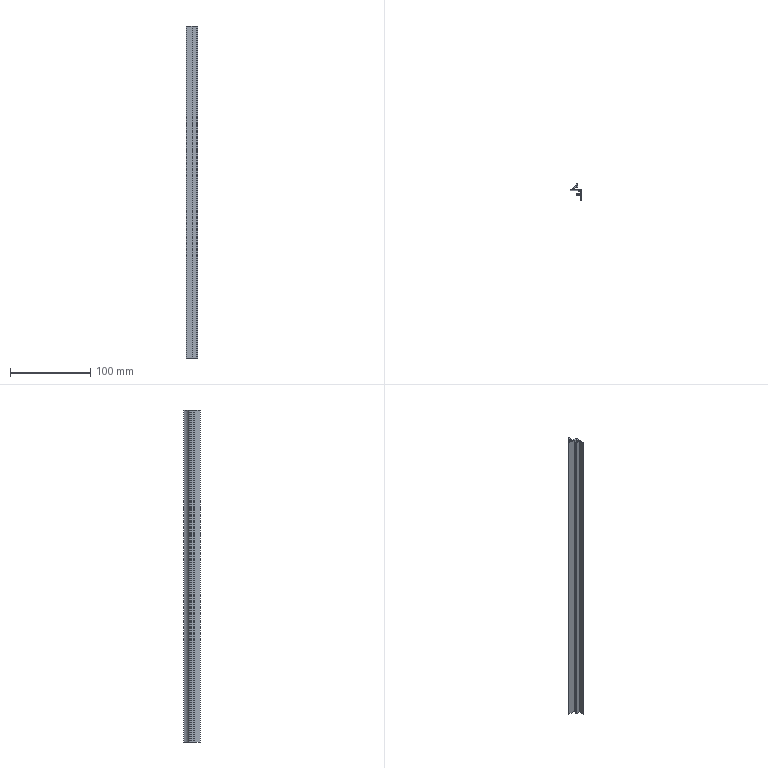Part | SolidWorks | features BaseBody 1, ICE 1, MoveFace 1 | 1 solid | 27 faces | box 14 x 20.3 x 413 mm | volume 21028 mm3 | plane 20 | cylinder 7 | commonest cylinder face diameters 0.387 x2 0.8 x2 0.4 x1 20 x1 22 x1
STEP:
#1=CARTESIAN_POINT('',(-5.304,-0.625,200.));
#2=VERTEX_POINT('',#1);
#3=CARTESIAN_POINT('',(-5.449,-0.8125,200.));
#4=VERTEX_POINT('',#3);
#5=CARTESIAN_POINT('',(-5.255,-0.8125,200.));
#6=DIRECTION('',(0.,0.,1.));
#7=DIRECTION('',(-1.,0.,0.));
#8=AXIS2_PLACEMENT_3D('',#5,#6,#7);
#9=CIRCLE('',#8,0.1937);
#10=EDGE_CURVE('',#2,#4,#9,.T.);
#11=ORIENTED_EDGE('',*,*,#10,.T.);
#12=CARTESIAN_POINT('',(-5.449,-0.8125,-213.));
#13=VERTEX_POINT('',#12);
#14=CARTESIAN_POINT('',(-5.449,-0.8125,230.));
#15=DIRECTION('',(0.,0.,-1.));
#16=VECTOR('',#15,1000.);
#17=LINE('',#14,#16);
#18=EDGE_CURVE('',#4,#13,#17,.T.);
#19=ORIENTED_EDGE('',*,*,#18,.T.);
#20=CARTESIAN_POINT('',(-5.304,-0.625,-213.));
#21=VERTEX_POINT('',#20);
#22=CARTESIAN_POINT('',(-5.255,-0.8125,-213.));
#23=DIRECTION('',(0.,0.,-1.));
#24=DIRECTION('',(1.,0.,0.));
#25=AXIS2_PLACEMENT_3D('',#22,#23,#24);
#26=CIRCLE('',#25,0.1937);
#27=EDGE_CURVE('',#13,#21,#26,.T.);
#28=ORIENTED_EDGE('',*,*,#27,.T.);
#29=CARTESIAN_POINT('',(-5.304,-0.625,230.));
#30=DIRECTION('',(0.,0.,-1.));
#31=VECTOR('',#30,1000.);
#32=LINE('',#29,#31);
#33=EDGE_CURVE('',#2,#21,#32,.T.);
#34=ORIENTED_EDGE('',*,*,#33,.F.);
#35=EDGE_LOOP('',(#11,#19,#28,#34));
#36=FACE_OUTER_BOUND('',#35,.T.);
#37=CARTESIAN_POINT('',(-5.255,-0.8125,230.));
#38=DIRECTION('',(0.,0.,-1.));
#39=DIRECTION('',(-1.,0.,0.));
#40=AXIS2_PLACEMENT_3D('',#37,#38,#39);
#41=CYLINDRICAL_SURFACE('',#40,0.1937);
#42=ADVANCED_FACE('',(#36),#41,.F.);
#43=CARTESIAN_POINT('',(5.,-1.,-213.));
#44=VERTEX_POINT('',#43);
#45=CARTESIAN_POINT('',(5.,-14.3,-213.));
#46=VERTEX_POINT('',#45);
#47=CARTESIAN_POINT('',(5.,29.623,-213.));
#48=DIRECTION('',(0.,-1.,0.));
#49=VECTOR('',#48,1000.);
#50=LINE('',#47,#49);
#51=EDGE_CURVE('',#44,#46,#50,.T.);
#52=ORIENTED_EDGE('',*,*,#51,.F.);
#53=CARTESIAN_POINT('',(5.,-1.,200.));
#54=VERTEX_POINT('',#53);
#55=CARTESIAN_POINT('',(5.,-1.,230.));
#56=DIRECTION('',(0.,0.,-1.));
#57=VECTOR('',#56,1000.);
#58=LINE('',#55,#57);
#59=EDGE_CURVE('',#54,#44,#58,.T.);
#60=ORIENTED_EDGE('',*,*,#59,.F.);
#61=CARTESIAN_POINT('',(5.,-14.3,200.));
#62=VERTEX_POINT('',#61);
#63=CARTESIAN_POINT('',(5.,-14.3,200.));
#64=DIRECTION('',(0.,1.,0.));
#65=VECTOR('',#64,1000.);
#66=LINE('',#63,#65);
#67=EDGE_CURVE('',#62,#54,#66,.T.);
#68=ORIENTED_EDGE('',*,*,#67,.F.);
#69=CARTESIAN_POINT('',(5.,-14.3,230.));
#70=DIRECTION('',(0.,0.,1.));
#71=VECTOR('',#70,1000.);
#72=LINE('',#69,#71);
#73=EDGE_CURVE('',#46,#62,#72,.T.);
#74=ORIENTED_EDGE('',*,*,#73,.F.);
#75=EDGE_LOOP('',(#52,#60,#68,#74));
#76=FACE_OUTER_BOUND('',#75,.T.);
#77=CARTESIAN_POINT('',(5.,-14.3,230.));
#78=DIRECTION('',(-1.,0.,0.));
#79=DIRECTION('',(0.,0.,1.));
#80=AXIS2_PLACEMENT_3D('',#77,#78,#79);
#81=PLANE('',#80);
#82=ADVANCED_FACE('',(#76),#81,.F.);
#83=CARTESIAN_POINT('',(-9.,-2.,-213.));
#84=VERTEX_POINT('',#83);
#85=CARTESIAN_POINT('',(-9.,-2.,200.));
#86=VERTEX_POINT('',#85);
#87=CARTESIAN_POINT('',(-9.,-2.,230.));
#88=DIRECTION('',(0.,0.,1.));
#89=VECTOR('',#88,1000.);
#90=LINE('',#87,#89);
#91=EDGE_CURVE('',#84,#86,#90,.T.);
#92=ORIENTED_EDGE('',*,*,#91,.F.);
#93=CARTESIAN_POINT('',(0.9,-2.,-213.));
#94=VERTEX_POINT('',#93);
#95=CARTESIAN_POINT('',(5.,-2.,-213.));
#96=DIRECTION('',(-1.,0.,0.));
#97=VECTOR('',#96,1000.);
#98=LINE('',#95,#97);
#99=EDGE_CURVE('',#94,#84,#98,.T.);
#100=ORIENTED_EDGE('',*,*,#99,.F.);
#101=CARTESIAN_POINT('',(0.9,-2.,200.));
#102=VERTEX_POINT('',#101);
#103=CARTESIAN_POINT('',(0.9,-2.,230.));
#104=DIRECTION('',(0.,0.,-1.));
#105=VECTOR('',#104,1000.);
#106=LINE('',#103,#105);
#107=EDGE_CURVE('',#102,#94,#106,.T.);
#108=ORIENTED_EDGE('',*,*,#107,.F.);
#109=CARTESIAN_POINT('',(5.,-2.,200.));
#110=DIRECTION('',(1.,0.,0.));
#111=VECTOR('',#110,1000.);
#112=LINE('',#109,#111);
#113=EDGE_CURVE('',#86,#102,#112,.T.);
#114=ORIENTED_EDGE('',*,*,#113,.F.);
#115=EDGE_LOOP('',(#92,#100,#108,#114));
#116=FACE_OUTER_BOUND('',#115,.T.);
#117=CARTESIAN_POINT('',(-9.,-2.,230.));
#118=DIRECTION('',(0.,1.,0.));
#119=DIRECTION('',(0.,0.,1.));
#120=AXIS2_PLACEMENT_3D('',#117,#118,#119);
#121=PLANE('',#120);
#122=ADVANCED_FACE('',(#116),#121,.F.);
#123=CARTESIAN_POINT('',(4.,-6.,200.));
#124=VERTEX_POINT('',#123);
#125=CARTESIAN_POINT('',(4.,-3.,200.));
#126=VERTEX_POINT('',#125);
#127=CARTESIAN_POINT('',(4.,29.623,200.));
#128=DIRECTION('',(0.,1.,0.));
#129=VECTOR('',#128,1000.);
#130=LINE('',#127,#129);
#131=EDGE_CURVE('',#124,#126,#130,.T.);
#132=ORIENTED_EDGE('',*,*,#131,.F.);
#133=CARTESIAN_POINT('',(1.,-6.,200.));
#134=VERTEX_POINT('',#133);
#135=CARTESIAN_POINT('',(5.,-6.,200.));
#136=DIRECTION('',(1.,0.,0.));
#137=VECTOR('',#136,1000.);
#138=LINE('',#135,#137);
#139=EDGE_CURVE('',#134,#124,#138,.T.);
#140=ORIENTED_EDGE('',*,*,#139,.F.);
#141=CARTESIAN_POINT('',(1.,-6.7,200.));
#142=VERTEX_POINT('',#141);
#143=CARTESIAN_POINT('',(1.,-6.,200.));
#144=DIRECTION('',(0.,-1.,0.));
#145=VECTOR('',#144,1000.);
#146=LINE('',#143,#145);
#147=EDGE_CURVE('',#134,#142,#146,.T.);
#148=ORIENTED_EDGE('',*,*,#147,.T.);
#149=CARTESIAN_POINT('',(-1.7,-6.7,200.));
#150=VERTEX_POINT('',#149);
#151=CARTESIAN_POINT('',(5.,-6.7,200.));
#152=DIRECTION('',(1.,0.,0.));
#153=VECTOR('',#152,1000.);
#154=LINE('',#151,#153);
#155=EDGE_CURVE('',#150,#142,#154,.T.);
#156=ORIENTED_EDGE('',*,*,#155,.F.);
#157=CARTESIAN_POINT('',(-1.7,-7.7,200.));
#158=VERTEX_POINT('',#157);
#159=CARTESIAN_POINT('',(-1.7,-6.7,200.));
#160=DIRECTION('',(0.,-1.,0.));
#161=VECTOR('',#160,1000.);
#162=LINE('',#159,#161);
#163=EDGE_CURVE('',#150,#158,#162,.T.);
#164=ORIENTED_EDGE('',*,*,#163,.T.);
#165=CARTESIAN_POINT('',(4.,-7.7,200.));
#166=VERTEX_POINT('',#165);
#167=CARTESIAN_POINT('',(5.,-7.7,200.));
#168=DIRECTION('',(-1.,0.,0.));
#169=VECTOR('',#168,1000.);
#170=LINE('',#167,#169);
#171=EDGE_CURVE('',#166,#158,#170,.T.);
#172=ORIENTED_EDGE('',*,*,#171,.F.);
#173=CARTESIAN_POINT('',(4.,-14.3,200.));
#174=VERTEX_POINT('',#173);
#175=CARTESIAN_POINT('',(4.,29.623,200.));
#176=DIRECTION('',(0.,1.,0.));
#177=VECTOR('',#176,1000.);
#178=LINE('',#175,#177);
#179=EDGE_CURVE('',#174,#166,#178,.T.);
#180=ORIENTED_EDGE('',*,*,#179,.F.);
#181=CARTESIAN_POINT('',(5.,-14.3,200.));
#182=DIRECTION('',(-1.,0.,0.));
#183=VECTOR('',#182,1000.);
#184=LINE('',#181,#183);
#185=EDGE_CURVE('',#62,#174,#184,.T.);
#186=ORIENTED_EDGE('',*,*,#185,.F.);
#187=ORIENTED_EDGE('',*,*,#67,.T.);
#188=CARTESIAN_POINT('',(-5.207,-1.,200.));
#189=VERTEX_POINT('',#188);
#190=CARTESIAN_POINT('',(5.,-1.,200.));
#191=DIRECTION('',(1.,0.,0.));
#192=VECTOR('',#191,1000.);
#193=LINE('',#190,#192);
#194=EDGE_CURVE('',#189,#54,#193,.T.);
#195=ORIENTED_EDGE('',*,*,#194,.F.);
#196=CARTESIAN_POINT('',(-5.255,-0.8125,200.));
#197=DIRECTION('',(0.,0.,1.));
#198=DIRECTION('',(-1.,0.,0.));
#199=AXIS2_PLACEMENT_3D('',#196,#197,#198);
#200=CIRCLE('',#199,0.1937);
#201=EDGE_CURVE('',#4,#189,#200,.T.);
#202=ORIENTED_EDGE('',*,*,#201,.F.);
#203=ORIENTED_EDGE('',*,*,#10,.F.);
#204=CARTESIAN_POINT('',(-1.368,3.063,200.));
#205=VERTEX_POINT('',#204);
#206=CARTESIAN_POINT('',(-10.628,9.,200.));
#207=DIRECTION('',(0.,0.,1.));
#208=DIRECTION('',(-1.,0.,0.));
#209=AXIS2_PLACEMENT_3D('',#206,#207,#208);
#210=CIRCLE('',#209,11.);
#211=EDGE_CURVE('',#2,#205,#210,.T.);
#212=ORIENTED_EDGE('',*,*,#211,.T.);
#213=CARTESIAN_POINT('',(-1.,2.955,200.));
#214=VERTEX_POINT('',#213);
#215=CARTESIAN_POINT('',(-1.2,2.955,200.));
#216=DIRECTION('',(0.,0.,1.));
#217=DIRECTION('',(-1.,0.,0.));
#218=AXIS2_PLACEMENT_3D('',#215,#216,#217);
#219=CIRCLE('',#218,0.2);
#220=EDGE_CURVE('',#214,#205,#219,.T.);
#221=ORIENTED_EDGE('',*,*,#220,.F.);
#222=CARTESIAN_POINT('',(-1.,1.5,200.));
#223=VERTEX_POINT('',#222);
#224=CARTESIAN_POINT('',(-1.,2.955,200.));
#225=DIRECTION('',(0.,1.,0.));
#226=VECTOR('',#225,1000.);
#227=LINE('',#224,#226);
#228=EDGE_CURVE('',#223,#214,#227,.T.);
#229=ORIENTED_EDGE('',*,*,#228,.F.);
#230=CARTESIAN_POINT('',(0.,1.5,200.));
#231=VERTEX_POINT('',#230);
#232=CARTESIAN_POINT('',(-1.,1.5,200.));
#233=DIRECTION('',(-1.,0.,0.));
#234=VECTOR('',#233,1000.);
#235=LINE('',#232,#234);
#236=EDGE_CURVE('',#231,#223,#235,.T.);
#237=ORIENTED_EDGE('',*,*,#236,.F.);
#238=CARTESIAN_POINT('',(0.,6.,200.));
#239=VERTEX_POINT('',#238);
#240=CARTESIAN_POINT('',(0.,1.5,200.));
#241=DIRECTION('',(0.,-1.,0.));
#242=VECTOR('',#241,1000.);
#243=LINE('',#240,#242);
#244=EDGE_CURVE('',#239,#231,#243,.T.);
#245=ORIENTED_EDGE('',*,*,#244,.F.);
#246=CARTESIAN_POINT('',(-0.8,6.,200.));
#247=VERTEX_POINT('',#246);
#248=CARTESIAN_POINT('',(0.,6.,200.));
#249=DIRECTION('',(1.,0.,0.));
#250=VECTOR('',#249,1000.);
#251=LINE('',#248,#250);
#252=EDGE_CURVE('',#247,#239,#251,.T.);
#253=ORIENTED_EDGE('',*,*,#252,.F.);
#254=CARTESIAN_POINT('',(-1.178,5.731,200.));
#255=VERTEX_POINT('',#254);
#256=CARTESIAN_POINT('',(-0.8,5.6,200.));
#257=DIRECTION('',(0.,0.,1.));
#258=DIRECTION('',(-1.,0.,0.));
#259=AXIS2_PLACEMENT_3D('',#256,#257,#258);
#260=CIRCLE('',#259,0.4);
#261=EDGE_CURVE('',#247,#255,#260,.T.);
#262=ORIENTED_EDGE('',*,*,#261,.T.);
#263=CARTESIAN_POINT('',(-8.678,-0.8077,200.));
#264=VERTEX_POINT('',#263);
#265=CARTESIAN_POINT('',(-10.628,9.,200.));
#266=DIRECTION('',(0.,0.,1.));
#267=DIRECTION('',(-1.,0.,0.));
#268=AXIS2_PLACEMENT_3D('',#265,#266,#267);
#269=CIRCLE('',#268,10.);
#270=EDGE_CURVE('',#264,#255,#269,.T.);
#271=ORIENTED_EDGE('',*,*,#270,.F.);
#272=CARTESIAN_POINT('',(-9.,-1.2,200.));
#273=VERTEX_POINT('',#272);
#274=CARTESIAN_POINT('',(-8.6,-1.2,200.));
#275=DIRECTION('',(0.,0.,1.));
#276=DIRECTION('',(-1.,0.,0.));
#277=AXIS2_PLACEMENT_3D('',#274,#275,#276);
#278=CIRCLE('',#277,0.4);
#279=EDGE_CURVE('',#264,#273,#278,.T.);
#280=ORIENTED_EDGE('',*,*,#279,.T.);
#281=CARTESIAN_POINT('',(-9.,8.,200.));
#282=DIRECTION('',(0.,-1.,0.));
#283=VECTOR('',#282,1000.);
#284=LINE('',#281,#283);
#285=EDGE_CURVE('',#273,#86,#284,.T.);
#286=ORIENTED_EDGE('',*,*,#285,.T.);
#287=ORIENTED_EDGE('',*,*,#113,.T.);
#288=CARTESIAN_POINT('',(0.9,-3.,200.));
#289=VERTEX_POINT('',#288);
#290=CARTESIAN_POINT('',(0.9,29.623,200.));
#291=DIRECTION('',(0.,1.,0.));
#292=VECTOR('',#291,1000.);
#293=LINE('',#290,#292);
#294=EDGE_CURVE('',#289,#102,#293,.T.);
#295=ORIENTED_EDGE('',*,*,#294,.F.);
#296=CARTESIAN_POINT('',(5.,-3.,200.));
#297=DIRECTION('',(-1.,0.,0.));
#298=VECTOR('',#297,1000.);
#299=LINE('',#296,#298);
#300=EDGE_CURVE('',#126,#289,#299,.T.);
#301=ORIENTED_EDGE('',*,*,#300,.F.);
#302=EDGE_LOOP('',(#132,#140,#148,#156,#164,#172,#180,#186,#187,#195,#202,#203,#212,#221,#229,#237,#245,#253,#262,#271,#280,#286,#287,#295,#301));
#303=FACE_OUTER_BOUND('',#302,.T.);
#304=CARTESIAN_POINT('',(5.,29.623,200.));
#305=DIRECTION('',(0.,0.,-1.));
#306=DIRECTION('',(-1.,0.,0.));
#307=AXIS2_PLACEMENT_3D('',#304,#305,#306);
#308=PLANE('',#307);
#309=ADVANCED_FACE('',(#303),#308,.F.);
#310=ORIENTED_EDGE('',*,*,#185,.T.);
#311=CARTESIAN_POINT('',(4.,-14.3,-213.));
#312=VERTEX_POINT('',#311);
#313=CARTESIAN_POINT('',(4.,-14.3,230.));
#314=DIRECTION('',(0.,0.,1.));
#315=VECTOR('',#314,1000.);
#316=LINE('',#313,#315);
#317=EDGE_CURVE('',#312,#174,#316,.T.);
#318=ORIENTED_EDGE('',*,*,#317,.F.);
#319=CARTESIAN_POINT('',(5.,-14.3,-213.));
#320=DIRECTION('',(-1.,0.,0.));
#321=VECTOR('',#320,1000.);
#322=LINE('',#319,#321);
#323=EDGE_CURVE('',#46,#312,#322,.T.);
#324=ORIENTED_EDGE('',*,*,#323,.F.);
#325=ORIENTED_EDGE('',*,*,#73,.T.);
#326=EDGE_LOOP('',(#310,#318,#324,#325));
#327=FACE_OUTER_BOUND('',#326,.T.);
#328=CARTESIAN_POINT('',(4.,-14.3,230.));
#329=DIRECTION('',(0.,1.,0.));
#330=DIRECTION('',(0.,0.,1.));
#331=AXIS2_PLACEMENT_3D('',#328,#329,#330);
#332=PLANE('',#331);
#333=ADVANCED_FACE('',(#327),#332,.F.);
#334=ORIENTED_EDGE('',*,*,#51,.T.);
#335=ORIENTED_EDGE('',*,*,#323,.T.);
#336=CARTESIAN_POINT('',(4.,-7.7,-213.));
#337=VERTEX_POINT('',#336);
#338=CARTESIAN_POINT('',(4.,-7.7,-213.));
#339=DIRECTION('',(0.,-1.,0.));
#340=VECTOR('',#339,1000.);
#341=LINE('',#338,#340);
#342=EDGE_CURVE('',#337,#312,#341,.T.);
#343=ORIENTED_EDGE('',*,*,#342,.F.);
#344=CARTESIAN_POINT('',(-1.7,-7.7,-213.));
#345=VERTEX_POINT('',#344);
#346=CARTESIAN_POINT('',(-1.7,-7.7,-213.));
#347=DIRECTION('',(1.,0.,0.));
#348=VECTOR('',#347,1000.);
#349=LINE('',#346,#348);
#350=EDGE_CURVE('',#345,#337,#349,.T.);
#351=ORIENTED_EDGE('',*,*,#350,.F.);
#352=CARTESIAN_POINT('',(-1.7,-6.7,-213.));
#353=VERTEX_POINT('',#352);
#354=CARTESIAN_POINT('',(-1.7,29.623,-213.));
#355=DIRECTION('',(0.,1.,0.));
#356=VECTOR('',#355,1000.);
#357=LINE('',#354,#356);
#358=EDGE_CURVE('',#345,#353,#357,.T.);
#359=ORIENTED_EDGE('',*,*,#358,.T.);
#360=CARTESIAN_POINT('',(1.,-6.7,-213.));
#361=VERTEX_POINT('',#360);
#362=CARTESIAN_POINT('',(1.,-6.7,-213.));
#363=DIRECTION('',(-1.,0.,0.));
#364=VECTOR('',#363,1000.);
#365=LINE('',#362,#364);
#366=EDGE_CURVE('',#361,#353,#365,.T.);
#367=ORIENTED_EDGE('',*,*,#366,.F.);
#368=CARTESIAN_POINT('',(1.,-6.,-213.));
#369=VERTEX_POINT('',#368);
#370=CARTESIAN_POINT('',(1.,29.623,-213.));
#371=DIRECTION('',(0.,1.,0.));
#372=VECTOR('',#371,1000.);
#373=LINE('',#370,#372);
#374=EDGE_CURVE('',#361,#369,#373,.T.);
#375=ORIENTED_EDGE('',*,*,#374,.T.);
#376=CARTESIAN_POINT('',(4.,-6.,-213.));
#377=VERTEX_POINT('',#376);
#378=CARTESIAN_POINT('',(4.,-6.,-213.));
#379=DIRECTION('',(-1.,0.,0.));
#380=VECTOR('',#379,1000.);
#381=LINE('',#378,#380);
#382=EDGE_CURVE('',#377,#369,#381,.T.);
#383=ORIENTED_EDGE('',*,*,#382,.F.);
#384=CARTESIAN_POINT('',(4.,-3.,-213.));
#385=VERTEX_POINT('',#384);
#386=CARTESIAN_POINT('',(4.,-3.,-213.));
#387=DIRECTION('',(0.,-1.,0.));
#388=VECTOR('',#387,1000.);
#389=LINE('',#386,#388);
#390=EDGE_CURVE('',#385,#377,#389,.T.);
#391=ORIENTED_EDGE('',*,*,#390,.F.);
#392=CARTESIAN_POINT('',(0.9,-3.,-213.));
#393=VERTEX_POINT('',#392);
#394=CARTESIAN_POINT('',(0.9,-3.,-213.));
#395=DIRECTION('',(1.,0.,0.));
#396=VECTOR('',#395,1000.);
#397=LINE('',#394,#396);
#398=EDGE_CURVE('',#393,#385,#397,.T.);
#399=ORIENTED_EDGE('',*,*,#398,.F.);
#400=CARTESIAN_POINT('',(0.9,-2.,-213.));
#401=DIRECTION('',(0.,-1.,0.));
#402=VECTOR('',#401,1000.);
#403=LINE('',#400,#402);
#404=EDGE_CURVE('',#94,#393,#403,.T.);
#405=ORIENTED_EDGE('',*,*,#404,.F.);
#406=ORIENTED_EDGE('',*,*,#99,.T.);
#407=CARTESIAN_POINT('',(-9.,-1.2,-213.));
#408=VERTEX_POINT('',#407);
#409=CARTESIAN_POINT('',(-9.,-1.2,-213.));
#410=DIRECTION('',(0.,-1.,0.));
#411=VECTOR('',#410,1000.);
#412=LINE('',#409,#411);
#413=EDGE_CURVE('',#408,#84,#412,.T.);
#414=ORIENTED_EDGE('',*,*,#413,.F.);
#415=CARTESIAN_POINT('',(-8.678,-0.8077,-213.));
#416=VERTEX_POINT('',#415);
#417=CARTESIAN_POINT('',(-8.6,-1.2,-213.));
#418=DIRECTION('',(0.,0.,-1.));
#419=DIRECTION('',(1.,0.,0.));
#420=AXIS2_PLACEMENT_3D('',#417,#418,#419);
#421=CIRCLE('',#420,0.4);
#422=EDGE_CURVE('',#408,#416,#421,.T.);
#423=ORIENTED_EDGE('',*,*,#422,.T.);
#424=CARTESIAN_POINT('',(-1.178,5.731,-213.));
#425=VERTEX_POINT('',#424);
#426=CARTESIAN_POINT('',(-10.628,9.,-213.));
#427=DIRECTION('',(0.,0.,-1.));
#428=DIRECTION('',(1.,0.,0.));
#429=AXIS2_PLACEMENT_3D('',#426,#427,#428);
#430=CIRCLE('',#429,10.);
#431=EDGE_CURVE('',#425,#416,#430,.T.);
#432=ORIENTED_EDGE('',*,*,#431,.F.);
#433=CARTESIAN_POINT('',(-0.8,6.,-213.));
#434=VERTEX_POINT('',#433);
#435=CARTESIAN_POINT('',(-0.8,5.6,-213.));
#436=DIRECTION('',(0.,0.,-1.));
#437=DIRECTION('',(1.,0.,0.));
#438=AXIS2_PLACEMENT_3D('',#435,#436,#437);
#439=CIRCLE('',#438,0.4);
#440=EDGE_CURVE('',#425,#434,#439,.T.);
#441=ORIENTED_EDGE('',*,*,#440,.T.);
#442=CARTESIAN_POINT('',(0.,6.,-213.));
#443=VERTEX_POINT('',#442);
#444=CARTESIAN_POINT('',(0.,6.,-213.));
#445=DIRECTION('',(-1.,0.,0.));
#446=VECTOR('',#445,1000.);
#447=LINE('',#444,#446);
#448=EDGE_CURVE('',#443,#434,#447,.T.);
#449=ORIENTED_EDGE('',*,*,#448,.F.);
#450=CARTESIAN_POINT('',(0.,1.5,-213.));
#451=VERTEX_POINT('',#450);
#452=CARTESIAN_POINT('',(0.,1.5,-213.));
#453=DIRECTION('',(0.,1.,0.));
#454=VECTOR('',#453,1000.);
#455=LINE('',#452,#454);
#456=EDGE_CURVE('',#451,#443,#455,.T.);
#457=ORIENTED_EDGE('',*,*,#456,.F.);
#458=CARTESIAN_POINT('',(-1.,1.5,-213.));
#459=VERTEX_POINT('',#458);
#460=CARTESIAN_POINT('',(-1.,1.5,-213.));
#461=DIRECTION('',(1.,0.,0.));
#462=VECTOR('',#461,1000.);
#463=LINE('',#460,#462);
#464=EDGE_CURVE('',#459,#451,#463,.T.);
#465=ORIENTED_EDGE('',*,*,#464,.F.);
#466=CARTESIAN_POINT('',(-1.,2.955,-213.));
#467=VERTEX_POINT('',#466);
#468=CARTESIAN_POINT('',(-1.,2.955,-213.));
#469=DIRECTION('',(0.,-1.,0.));
#470=VECTOR('',#469,1000.);
#471=LINE('',#468,#470);
#472=EDGE_CURVE('',#467,#459,#471,.T.);
#473=ORIENTED_EDGE('',*,*,#472,.F.);
#474=CARTESIAN_POINT('',(-1.368,3.063,-213.));
#475=VERTEX_POINT('',#474);
#476=CARTESIAN_POINT('',(-1.2,2.955,-213.));
#477=DIRECTION('',(0.,0.,-1.));
#478=DIRECTION('',(1.,0.,0.));
#479=AXIS2_PLACEMENT_3D('',#476,#477,#478);
#480=CIRCLE('',#479,0.2);
#481=EDGE_CURVE('',#475,#467,#480,.T.);
#482=ORIENTED_EDGE('',*,*,#481,.F.);
#483=CARTESIAN_POINT('',(-10.628,9.,-213.));
#484=DIRECTION('',(0.,0.,-1.));
#485=DIRECTION('',(1.,0.,0.));
#486=AXIS2_PLACEMENT_3D('',#483,#484,#485);
#487=CIRCLE('',#486,11.);
#488=EDGE_CURVE('',#475,#21,#487,.T.);
#489=ORIENTED_EDGE('',*,*,#488,.T.);
#490=ORIENTED_EDGE('',*,*,#27,.F.);
#491=CARTESIAN_POINT('',(-5.207,-1.,-213.));
#492=VERTEX_POINT('',#491);
#493=CARTESIAN_POINT('',(-5.255,-0.8125,-213.));
#494=DIRECTION('',(0.,0.,-1.));
#495=DIRECTION('',(1.,0.,0.));
#496=AXIS2_PLACEMENT_3D('',#493,#494,#495);
#497=CIRCLE('',#496,0.1937);
#498=EDGE_CURVE('',#492,#13,#497,.T.);
#499=ORIENTED_EDGE('',*,*,#498,.F.);
#500=CARTESIAN_POINT('',(5.,-1.,-213.));
#501=DIRECTION('',(-1.,0.,0.));
#502=VECTOR('',#501,1000.);
#503=LINE('',#500,#502);
#504=EDGE_CURVE('',#44,#492,#503,.T.);
#505=ORIENTED_EDGE('',*,*,#504,.F.);
#506=EDGE_LOOP('',(#334,#335,#343,#351,#359,#367,#375,#383,#391,#399,#405,#406,#414,#423,#432,#441,#449,#457,#465,#473,#482,#489,#490,#499,#505));
#507=FACE_OUTER_BOUND('',#506,.T.);
#508=CARTESIAN_POINT('',(5.,29.623,-213.));
#509=DIRECTION('',(0.,0.,1.));
#510=DIRECTION('',(1.,0.,0.));
#511=AXIS2_PLACEMENT_3D('',#508,#509,#510);
#512=PLANE('',#511);
#513=ADVANCED_FACE('',(#507),#512,.F.);
#514=ORIENTED_EDGE('',*,*,#59,.T.);
#515=ORIENTED_EDGE('',*,*,#504,.T.);
#516=CARTESIAN_POINT('',(-5.207,-1.,230.));
#517=DIRECTION('',(0.,0.,-1.));
#518=VECTOR('',#517,1000.);
#519=LINE('',#516,#518);
#520=EDGE_CURVE('',#189,#492,#519,.T.);
#521=ORIENTED_EDGE('',*,*,#520,.F.);
#522=ORIENTED_EDGE('',*,*,#194,.T.);
#523=EDGE_LOOP('',(#514,#515,#521,#522));
#524=FACE_OUTER_BOUND('',#523,.T.);
#525=CARTESIAN_POINT('',(5.,-1.,230.));
#526=DIRECTION('',(0.,-1.,0.));
#527=DIRECTION('',(0.,0.,-1.));
#528=AXIS2_PLACEMENT_3D('',#525,#526,#527);
#529=PLANE('',#528);
#530=ADVANCED_FACE('',(#524),#529,.F.);
#531=CARTESIAN_POINT('',(-9.,-1.2,230.));
#532=DIRECTION('',(0.,0.,1.));
#533=VECTOR('',#532,1000.);
#534=LINE('',#531,#533);
#535=EDGE_CURVE('',#408,#273,#534,.T.);
#536=ORIENTED_EDGE('',*,*,#535,.F.);
#537=ORIENTED_EDGE('',*,*,#413,.T.);
#538=ORIENTED_EDGE('',*,*,#91,.T.);
#539=ORIENTED_EDGE('',*,*,#285,.F.);
#540=EDGE_LOOP('',(#536,#537,#538,#539));
#541=FACE_OUTER_BOUND('',#540,.T.);
#542=CARTESIAN_POINT('',(-9.,-1.2,230.));
#543=DIRECTION('',(1.,0.,0.));
#544=DIRECTION('',(0.,0.,-1.));
#545=AXIS2_PLACEMENT_3D('',#542,#543,#544);
#546=PLANE('',#545);
#547=ADVANCED_FACE('',(#541),#546,.F.);
#548=ORIENTED_EDGE('',*,*,#294,.T.);
#549=ORIENTED_EDGE('',*,*,#107,.T.);
#550=ORIENTED_EDGE('',*,*,#404,.T.);
#551=CARTESIAN_POINT('',(0.9,-3.,230.));
#552=DIRECTION('',(0.,0.,-1.));
#553=VECTOR('',#552,1000.);
#554=LINE('',#551,#553);
#555=EDGE_CURVE('',#289,#393,#554,.T.);
#556=ORIENTED_EDGE('',*,*,#555,.F.);
#557=EDGE_LOOP('',(#548,#549,#550,#556));
#558=FACE_OUTER_BOUND('',#557,.T.);
#559=CARTESIAN_POINT('',(0.9,-2.,230.));
#560=DIRECTION('',(1.,0.,0.));
#561=DIRECTION('',(0.,0.,-1.));
#562=AXIS2_PLACEMENT_3D('',#559,#560,#561);
#563=PLANE('',#562);
#564=ADVANCED_FACE('',(#558),#563,.F.);
#565=ORIENTED_EDGE('',*,*,#300,.T.);
#566=ORIENTED_EDGE('',*,*,#555,.T.);
#567=ORIENTED_EDGE('',*,*,#398,.T.);
#568=CARTESIAN_POINT('',(4.,-3.,230.));
#569=DIRECTION('',(0.,0.,-1.));
#570=VECTOR('',#569,1000.);
#571=LINE('',#568,#570);
#572=EDGE_CURVE('',#126,#385,#571,.T.);
#573=ORIENTED_EDGE('',*,*,#572,.F.);
#574=EDGE_LOOP('',(#565,#566,#567,#573));
#575=FACE_OUTER_BOUND('',#574,.T.);
#576=CARTESIAN_POINT('',(0.9,-3.,230.));
#577=DIRECTION('',(0.,1.,0.));
#578=DIRECTION('',(0.,0.,1.));
#579=AXIS2_PLACEMENT_3D('',#576,#577,#578);
#580=PLANE('',#579);
#581=ADVANCED_FACE('',(#575),#580,.F.);
#582=ORIENTED_EDGE('',*,*,#131,.T.);
#583=ORIENTED_EDGE('',*,*,#572,.T.);
#584=ORIENTED_EDGE('',*,*,#390,.T.);
#585=CARTESIAN_POINT('',(4.,-6.,230.));
#586=DIRECTION('',(0.,0.,-1.));
#587=VECTOR('',#586,1000.);
#588=LINE('',#585,#587);
#589=EDGE_CURVE('',#124,#377,#588,.T.);
#590=ORIENTED_EDGE('',*,*,#589,.F.);
#591=EDGE_LOOP('',(#582,#583,#584,#590));
#592=FACE_OUTER_BOUND('',#591,.T.);
#593=CARTESIAN_POINT('',(4.,-3.,230.));
#594=DIRECTION('',(1.,0.,0.));
#595=DIRECTION('',(0.,0.,-1.));
#596=AXIS2_PLACEMENT_3D('',#593,#594,#595);
#597=PLANE('',#596);
#598=ADVANCED_FACE('',(#592),#597,.F.);
#599=ORIENTED_EDGE('',*,*,#139,.T.);
#600=ORIENTED_EDGE('',*,*,#589,.T.);
#601=ORIENTED_EDGE('',*,*,#382,.T.);
#602=CARTESIAN_POINT('',(1.,-6.,230.));
#603=DIRECTION('',(0.,0.,-1.));
#604=VECTOR('',#603,1000.);
#605=LINE('',#602,#604);
#606=EDGE_CURVE('',#134,#369,#605,.T.);
#607=ORIENTED_EDGE('',*,*,#606,.F.);
#608=EDGE_LOOP('',(#599,#600,#601,#607));
#609=FACE_OUTER_BOUND('',#608,.T.);
#610=CARTESIAN_POINT('',(4.,-6.,230.));
#611=DIRECTION('',(0.,-1.,0.));
#612=DIRECTION('',(0.,0.,-1.));
#613=AXIS2_PLACEMENT_3D('',#610,#611,#612);
#614=PLANE('',#613);
#615=ADVANCED_FACE('',(#609),#614,.F.);
#616=ORIENTED_EDGE('',*,*,#155,.T.);
#617=CARTESIAN_POINT('',(1.,-6.7,230.));
#618=DIRECTION('',(0.,0.,1.));
#619=VECTOR('',#618,1000.);
#620=LINE('',#617,#619);
#621=EDGE_CURVE('',#361,#142,#620,.T.);
#622=ORIENTED_EDGE('',*,*,#621,.F.);
#623=ORIENTED_EDGE('',*,*,#366,.T.);
#624=CARTESIAN_POINT('',(-1.7,-6.7,230.));
#625=DIRECTION('',(0.,0.,-1.));
#626=VECTOR('',#625,1000.);
#627=LINE('',#624,#626);
#628=EDGE_CURVE('',#150,#353,#627,.T.);
#629=ORIENTED_EDGE('',*,*,#628,.F.);
#630=EDGE_LOOP('',(#616,#622,#623,#629));
#631=FACE_OUTER_BOUND('',#630,.T.);
#632=CARTESIAN_POINT('',(1.,-6.7,230.));
#633=DIRECTION('',(0.,-1.,0.));
#634=DIRECTION('',(0.,0.,-1.));
#635=AXIS2_PLACEMENT_3D('',#632,#633,#634);
#636=PLANE('',#635);
#637=ADVANCED_FACE('',(#631),#636,.F.);
#638=ORIENTED_EDGE('',*,*,#171,.T.);
#639=CARTESIAN_POINT('',(-1.7,-7.7,230.));
#640=DIRECTION('',(0.,0.,1.));
#641=VECTOR('',#640,1000.);
#642=LINE('',#639,#641);
#643=EDGE_CURVE('',#345,#158,#642,.T.);
#644=ORIENTED_EDGE('',*,*,#643,.F.);
#645=ORIENTED_EDGE('',*,*,#350,.T.);
#646=CARTESIAN_POINT('',(4.,-7.7,230.));
#647=DIRECTION('',(0.,0.,-1.));
#648=VECTOR('',#647,1000.);
#649=LINE('',#646,#648);
#650=EDGE_CURVE('',#166,#337,#649,.T.);
#651=ORIENTED_EDGE('',*,*,#650,.F.);
#652=EDGE_LOOP('',(#638,#644,#645,#651));
#653=FACE_OUTER_BOUND('',#652,.T.);
#654=CARTESIAN_POINT('',(-1.7,-7.7,230.));
#655=DIRECTION('',(0.,1.,0.));
#656=DIRECTION('',(0.,0.,1.));
#657=AXIS2_PLACEMENT_3D('',#654,#655,#656);
#658=PLANE('',#657);
#659=ADVANCED_FACE('',(#653),#658,.F.);
#660=ORIENTED_EDGE('',*,*,#179,.T.);
#661=ORIENTED_EDGE('',*,*,#650,.T.);
#662=ORIENTED_EDGE('',*,*,#342,.T.);
#663=ORIENTED_EDGE('',*,*,#317,.T.);
#664=EDGE_LOOP('',(#660,#661,#662,#663));
#665=FACE_OUTER_BOUND('',#664,.T.);
#666=CARTESIAN_POINT('',(4.,-7.7,230.));
#667=DIRECTION('',(1.,0.,0.));
#668=DIRECTION('',(0.,0.,-1.));
#669=AXIS2_PLACEMENT_3D('',#666,#667,#668);
#670=PLANE('',#669);
#671=ADVANCED_FACE('',(#665),#670,.F.);
#672=ORIENTED_EDGE('',*,*,#18,.F.);
#673=ORIENTED_EDGE('',*,*,#201,.T.);
#674=ORIENTED_EDGE('',*,*,#520,.T.);
#675=ORIENTED_EDGE('',*,*,#498,.T.);
#676=EDGE_LOOP('',(#672,#673,#674,#675));
#677=FACE_OUTER_BOUND('',#676,.T.);
#678=CARTESIAN_POINT('',(-5.255,-0.8125,230.));
#679=DIRECTION('',(0.,0.,-1.));
#680=DIRECTION('',(-1.,0.,0.));
#681=AXIS2_PLACEMENT_3D('',#678,#679,#680);
#682=CYLINDRICAL_SURFACE('',#681,0.1937);
#683=ADVANCED_FACE('',(#677),#682,.F.);
#684=CARTESIAN_POINT('',(-1.,2.955,230.));
#685=DIRECTION('',(0.,0.,1.));
#686=VECTOR('',#685,1000.);
#687=LINE('',#684,#686);
#688=EDGE_CURVE('',#467,#214,#687,.T.);
#689=ORIENTED_EDGE('',*,*,#688,.F.);
#690=ORIENTED_EDGE('',*,*,#472,.T.);
#691=CARTESIAN_POINT('',(-1.,1.5,230.));
#692=DIRECTION('',(0.,0.,-1.));
#693=VECTOR('',#692,1000.);
#694=LINE('',#691,#693);
#695=EDGE_CURVE('',#223,#459,#694,.T.);
#696=ORIENTED_EDGE('',*,*,#695,.F.);
#697=ORIENTED_EDGE('',*,*,#228,.T.);
#698=EDGE_LOOP('',(#689,#690,#696,#697));
#699=FACE_OUTER_BOUND('',#698,.T.);
#700=CARTESIAN_POINT('',(-1.,2.955,230.));
#701=DIRECTION('',(1.,0.,0.));
#702=DIRECTION('',(0.,0.,-1.));
#703=AXIS2_PLACEMENT_3D('',#700,#701,#702);
#704=PLANE('',#703);
#705=ADVANCED_FACE('',(#699),#704,.F.);
#706=ORIENTED_EDGE('',*,*,#488,.F.);
#707=CARTESIAN_POINT('',(-1.368,3.063,230.));
#708=DIRECTION('',(0.,0.,1.));
#709=VECTOR('',#708,1000.);
#710=LINE('',#707,#709);
#711=EDGE_CURVE('',#475,#205,#710,.T.);
#712=ORIENTED_EDGE('',*,*,#711,.T.);
#713=ORIENTED_EDGE('',*,*,#211,.F.);
#714=ORIENTED_EDGE('',*,*,#33,.T.);
#715=EDGE_LOOP('',(#706,#712,#713,#714));
#716=FACE_OUTER_BOUND('',#715,.T.);
#717=CARTESIAN_POINT('',(-10.628,9.,230.));
#718=DIRECTION('',(0.,0.,-1.));
#719=DIRECTION('',(-1.,0.,0.));
#720=AXIS2_PLACEMENT_3D('',#717,#718,#719);
#721=CYLINDRICAL_SURFACE('',#720,11.);
#722=ADVANCED_FACE('',(#716),#721,.T.);
#723=CARTESIAN_POINT('',(-1.178,5.731,230.));
#724=DIRECTION('',(0.,0.,1.));
#725=VECTOR('',#724,1000.);
#726=LINE('',#723,#725);
#727=EDGE_CURVE('',#425,#255,#726,.T.);
#728=ORIENTED_EDGE('',*,*,#727,.F.);
#729=ORIENTED_EDGE('',*,*,#431,.T.);
#730=CARTESIAN_POINT('',(-8.678,-0.8077,230.));
#731=DIRECTION('',(0.,0.,-1.));
#732=VECTOR('',#731,1000.);
#733=LINE('',#730,#732);
#734=EDGE_CURVE('',#264,#416,#733,.T.);
#735=ORIENTED_EDGE('',*,*,#734,.F.);
#736=ORIENTED_EDGE('',*,*,#270,.T.);
#737=EDGE_LOOP('',(#728,#729,#735,#736));
#738=FACE_OUTER_BOUND('',#737,.T.);
#739=CARTESIAN_POINT('',(-10.628,9.,230.));
#740=DIRECTION('',(0.,0.,-1.));
#741=DIRECTION('',(-1.,0.,0.));
#742=AXIS2_PLACEMENT_3D('',#739,#740,#741);
#743=CYLINDRICAL_SURFACE('',#742,10.);
#744=ADVANCED_FACE('',(#738),#743,.F.);
#745=CARTESIAN_POINT('',(0.,1.5,230.));
#746=DIRECTION('',(0.,0.,1.));
#747=VECTOR('',#746,1000.);
#748=LINE('',#745,#747);
#749=EDGE_CURVE('',#451,#231,#748,.T.);
#750=ORIENTED_EDGE('',*,*,#749,.F.);
#751=ORIENTED_EDGE('',*,*,#456,.T.);
#752=CARTESIAN_POINT('',(0.,6.,230.));
#753=DIRECTION('',(0.,0.,-1.));
#754=VECTOR('',#753,1000.);
#755=LINE('',#752,#754);
#756=EDGE_CURVE('',#239,#443,#755,.T.);
#757=ORIENTED_EDGE('',*,*,#756,.F.);
#758=ORIENTED_EDGE('',*,*,#244,.T.);
#759=EDGE_LOOP('',(#750,#751,#757,#758));
#760=FACE_OUTER_BOUND('',#759,.T.);
#761=CARTESIAN_POINT('',(0.,1.5,230.));
#762=DIRECTION('',(-1.,0.,0.));
#763=DIRECTION('',(0.,0.,1.));
#764=AXIS2_PLACEMENT_3D('',#761,#762,#763);
#765=PLANE('',#764);
#766=ADVANCED_FACE('',(#760),#765,.F.);
#767=ORIENTED_EDGE('',*,*,#422,.F.);
#768=ORIENTED_EDGE('',*,*,#535,.T.);
#769=ORIENTED_EDGE('',*,*,#279,.F.);
#770=ORIENTED_EDGE('',*,*,#734,.T.);
#771=EDGE_LOOP('',(#767,#768,#769,#770));
#772=FACE_OUTER_BOUND('',#771,.T.);
#773=CARTESIAN_POINT('',(-8.6,-1.2,230.));
#774=DIRECTION('',(0.,0.,-1.));
#775=DIRECTION('',(-1.,0.,0.));
#776=AXIS2_PLACEMENT_3D('',#773,#774,#775);
#777=CYLINDRICAL_SURFACE('',#776,0.4);
#778=ADVANCED_FACE('',(#772),#777,.T.);
#779=ORIENTED_EDGE('',*,*,#147,.F.);
#780=ORIENTED_EDGE('',*,*,#606,.T.);
#781=ORIENTED_EDGE('',*,*,#374,.F.);
#782=ORIENTED_EDGE('',*,*,#621,.T.);
#783=EDGE_LOOP('',(#779,#780,#781,#782));
#784=FACE_OUTER_BOUND('',#783,.T.);
#785=CARTESIAN_POINT('',(1.,-6.,230.));
#786=DIRECTION('',(1.,0.,0.));
#787=DIRECTION('',(0.,0.,-1.));
#788=AXIS2_PLACEMENT_3D('',#785,#786,#787);
#789=PLANE('',#788);
#790=ADVANCED_FACE('',(#784),#789,.F.);
#791=ORIENTED_EDGE('',*,*,#163,.F.);
#792=ORIENTED_EDGE('',*,*,#628,.T.);
#793=ORIENTED_EDGE('',*,*,#358,.F.);
#794=ORIENTED_EDGE('',*,*,#643,.T.);
#795=EDGE_LOOP('',(#791,#792,#793,#794));
#796=FACE_OUTER_BOUND('',#795,.T.);
#797=CARTESIAN_POINT('',(-1.7,-6.7,230.));
#798=DIRECTION('',(1.,0.,0.));
#799=DIRECTION('',(0.,0.,-1.));
#800=AXIS2_PLACEMENT_3D('',#797,#798,#799);
#801=PLANE('',#800);
#802=ADVANCED_FACE('',(#796),#801,.F.);
#803=ORIENTED_EDGE('',*,*,#711,.F.);
#804=ORIENTED_EDGE('',*,*,#481,.T.);
#805=ORIENTED_EDGE('',*,*,#688,.T.);
#806=ORIENTED_EDGE('',*,*,#220,.T.);
#807=EDGE_LOOP('',(#803,#804,#805,#806));
#808=FACE_OUTER_BOUND('',#807,.T.);
#809=CARTESIAN_POINT('',(-1.2,2.955,230.));
#810=DIRECTION('',(0.,0.,-1.));
#811=DIRECTION('',(-1.,0.,0.));
#812=AXIS2_PLACEMENT_3D('',#809,#810,#811);
#813=CYLINDRICAL_SURFACE('',#812,0.2);
#814=ADVANCED_FACE('',(#808),#813,.F.);
#815=ORIENTED_EDGE('',*,*,#695,.T.);
#816=ORIENTED_EDGE('',*,*,#464,.T.);
#817=ORIENTED_EDGE('',*,*,#749,.T.);
#818=ORIENTED_EDGE('',*,*,#236,.T.);
#819=EDGE_LOOP('',(#815,#816,#817,#818));
#820=FACE_OUTER_BOUND('',#819,.T.);
#821=CARTESIAN_POINT('',(-1.,1.5,230.));
#822=DIRECTION('',(0.,1.,0.));
#823=DIRECTION('',(0.,0.,1.));
#824=AXIS2_PLACEMENT_3D('',#821,#822,#823);
#825=PLANE('',#824);
#826=ADVANCED_FACE('',(#820),#825,.F.);
#827=ORIENTED_EDGE('',*,*,#440,.F.);
#828=ORIENTED_EDGE('',*,*,#727,.T.);
#829=ORIENTED_EDGE('',*,*,#261,.F.);
#830=CARTESIAN_POINT('',(-0.8,6.,230.));
#831=DIRECTION('',(0.,0.,-1.));
#832=VECTOR('',#831,1000.);
#833=LINE('',#830,#832);
#834=EDGE_CURVE('',#247,#434,#833,.T.);
#835=ORIENTED_EDGE('',*,*,#834,.T.);
#836=EDGE_LOOP('',(#827,#828,#829,#835));
#837=FACE_OUTER_BOUND('',#836,.T.);
#838=CARTESIAN_POINT('',(-0.8,5.6,230.));
#839=DIRECTION('',(0.,0.,-1.));
#840=DIRECTION('',(-1.,0.,0.));
#841=AXIS2_PLACEMENT_3D('',#838,#839,#840);
#842=CYLINDRICAL_SURFACE('',#841,0.4);
#843=ADVANCED_FACE('',(#837),#842,.T.);
#844=ORIENTED_EDGE('',*,*,#756,.T.);
#845=ORIENTED_EDGE('',*,*,#448,.T.);
#846=ORIENTED_EDGE('',*,*,#834,.F.);
#847=ORIENTED_EDGE('',*,*,#252,.T.);
#848=EDGE_LOOP('',(#844,#845,#846,#847));
#849=FACE_OUTER_BOUND('',#848,.T.);
#850=CARTESIAN_POINT('',(0.,6.,230.));
#851=DIRECTION('',(0.,-1.,0.));
#852=DIRECTION('',(0.,0.,-1.));
#853=AXIS2_PLACEMENT_3D('',#850,#851,#852);
#854=PLANE('',#853);
#855=ADVANCED_FACE('',(#849),#854,.F.);
#856=CLOSED_SHELL('',(#42,#82,#122,#309,#333,#513,#530,#547,#564,#581,#598,#615,#637,#659,#671,#683,#705,#722,#744,#766,#778,#790,#802,#814,#826,#843,#855));
#857=MANIFOLD_SOLID_BREP('',#856);
#858=CARTESIAN_POINT('',(0.,0.,0.));
#859=DIRECTION('',(0.,0.,1.));
#860=DIRECTION('',(1.,0.,0.));
#861=AXIS2_PLACEMENT_3D('',#858,#859,#860);
#862=(LENGTH_UNIT()NAMED_UNIT(*)SI_UNIT(.MILLI.,.METRE.));
#863=UNCERTAINTY_MEASURE_WITH_UNIT(LENGTH_MEASURE(0.00001),#862,'','');
#864=(NAMED_UNIT(*)PLANE_ANGLE_UNIT()SI_UNIT($,.RADIAN.));
#865=(NAMED_UNIT(*)SI_UNIT($,.STERADIAN.)SOLID_ANGLE_UNIT());
#866=(GEOMETRIC_REPRESENTATION_CONTEXT(3)GLOBAL_UNCERTAINTY_ASSIGNED_CONTEXT((#863))GLOBAL_UNIT_ASSIGNED_CONTEXT((#862,#864,#865))REPRESENTATION_CONTEXT('',''));
#867=ADVANCED_BREP_SHAPE_REPRESENTATION('',(#857,#861),#866);